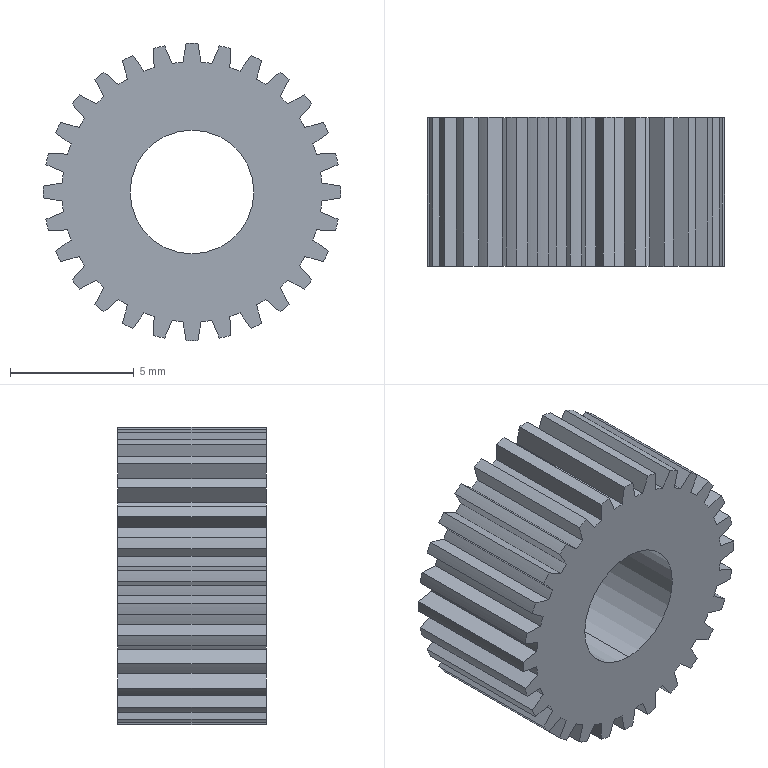Part | SolidWorks | features BaseBody 1 | 1 solid | 117 faces | box 12 x 6 x 12 mm | volume 478.272 mm3 | cylinder 59 | plane 58 | commonest cylinder face diameters 12 x29 10.5 x28 5 x2